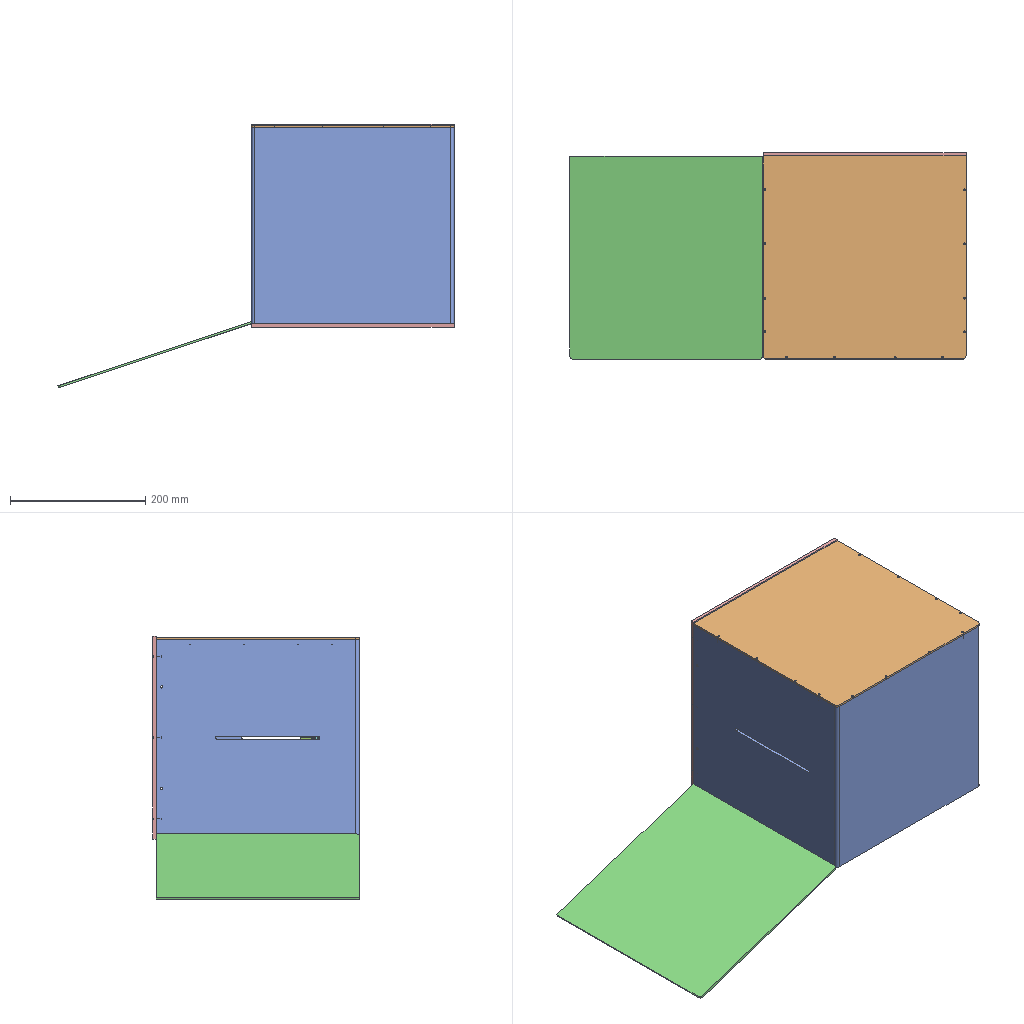Assembly | SolidWorks | 8 different items | 8 placed | box 586 x 305 x 390 mm
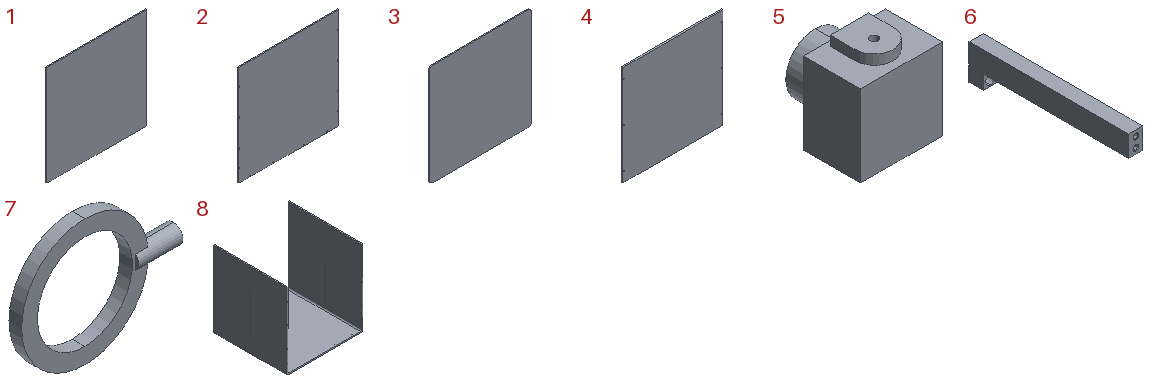Parts list (item | quantity | size | volume | features):
1 | x1 | 300 x 3 x 300 mm | 269968 mm3 | features Extrusion 1
2 | x1 | 300 x 3 x 300 mm | 269713 mm3 | features Extrusion 1
3 | x1 | 288 x 3 x 288 mm | 248574 mm3 | features Extrusion 1
4 | x1 | 300 x 5 x 300 mm | 449761 mm3 | features Extrusion 1, HoleWzd 1
5 | x1 | 50 x 53 x 56 mm | 108930 mm3 | features ICE 2, Extrusion 1, HoleWzd 1
6 | x1 | 10 x 114 x 25 mm | 17594 mm3 | features Extrusion 1, HoleWzd 1, ICE 1
7 | x1 | 250 x 30 x 200 mm | 313165 mm3 | features Extrusion 1, HoleWzd 1, ICE 1
8 | x1 | 300 x 290 x 300 mm | 1282164 mm3 | features HoleWzd 3, ICE 2, Extrusion 1
Mates (type | each side: item.copy, entity, surface, feature):
Coincident | 4.1 face plane Boss-Extrude1 | 8.1 face plane Boss-Extrude1
Concentric | 4.1 face cone CSK for M2.5 Flat Head Machine Screw1 | 8.1 face cylinder M2.5 Tapped Hole1 | 2 times
Concentric | 5.1 face cylinder M6 Tapped Hole1 | 6.1 face cylinder Boss-Extrude2
Coincident | 5.1 face plane Boss-Extrude3 | 6.1 face plane Boss-Extrude1
Parallel | 5.1 face plane Boss-Extrude1 | 6.1 face plane Boss-Extrude2
Coincident | 8.1 face plane Boss-Extrude1 | 6.1 face plane Boss-Extrude1
Concentric | 8.1 face cylinder Cut-Extrude2 | 6.1 face cylinder M4 Tapped Hole1
Parallel | 8.1 face plane Boss-Extrude1 | 5.1 face plane Boss-Extrude1
Coincident | 8.1 face plane Boss-Extrude1 | 7.1 face plane Boss-Extrude2
Coincident | 8.1 face plane Boss-Extrude1 | 2.1 face plane Boss-Extrude1
Concentric | 8.1 face cylinder M2.5 Tapped Hole2 | 2.1 face cylinder Boss-Extrude1 | 2 times
Parallel | 4.1 face plane Boss-Extrude1 | 3.1 face plane Boss-Extrude1
DistanceDim | 3.1 face plane Boss-Extrude1 | 8.1 face plane Boss-Extrude1
DistanceDim | 2.1 face plane Boss-Extrude1 | 3.1 face plane Boss-Extrude1
DistanceDim | 4.1 face plane Boss-Extrude1 | 3.1 face plane Boss-Extrude1
Coincident | 4.1 face plane Boss-Extrude1 | 1.1 face plane Boss-Extrude1
Coincident | 8.1 edge | 1.1 edge
Concentric | 8.1 face cylinder Cut-Extrude3 | 7.1 face cylinder M6 Tapped Hole1